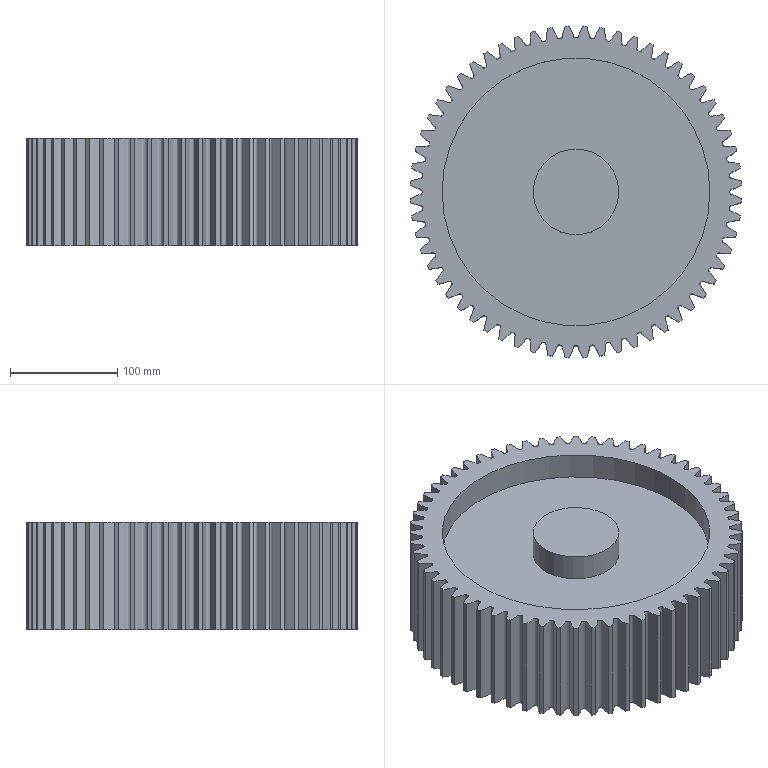Part | SolidWorks | 1 solid | 139 faces | box 309.756 x 309.756 x 100 mm | volume 4555207 mm3 | cylinder 70 | spline 60 | plane 9 | commonest cylinder face diameters 310 x60 80 x4 250 x4 40 x2